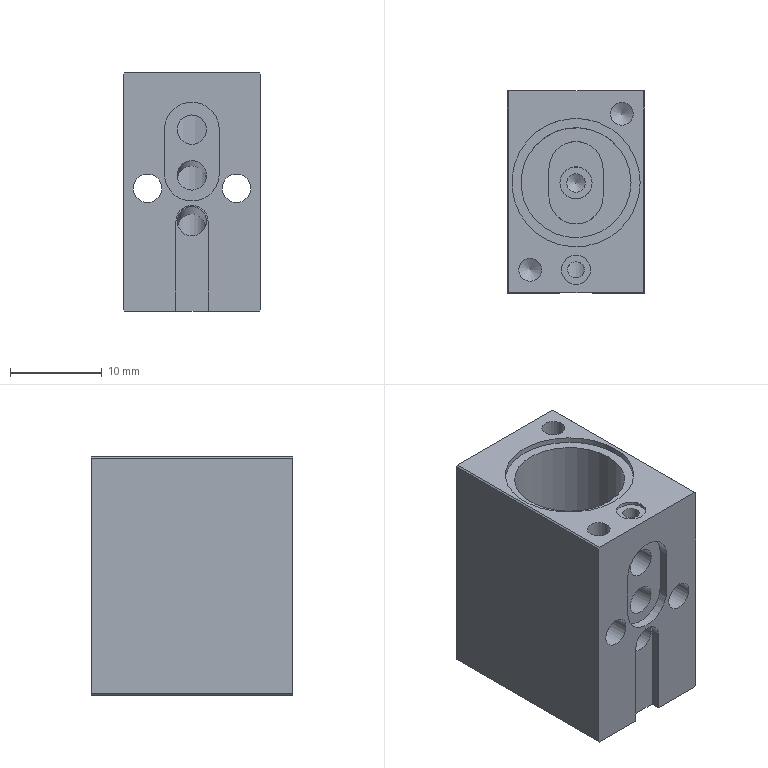NC program | NX | posted with a generic post | part box 15 x 22 x 26 mm
Whole program:
N10 G17 G21 G94 G90
(PLANAR_MILL_13 , TOOL : D8开粗)
N12 T13 M6
N14 G54
N16 G17 G0 G90 X-19. Y-18. B0. C0. S5500 M3
N18 G43 Z30. H13
N20 Z5.
N22 G94 G1 Z2. F1000.
N24 Y-10.
N26 Y10.
N28 Y18.
N30 Z5.
N32 G0 Z30.
N34 Y-18.
N36 Z4.
N38 G1 Z1.
N40 Y-10.
N42 Y10.
N44 Y18.
N46 Z4.
N48 G0 Z30.
N50 Y-18.
N52 Z3.
N54 G1 Z0.
N56 Y-10.
N58 Y10.
N60 Y18.
N62 Z3.
N64 G0 Z30.
(ADAPTIVE_MILLING_1 , TOOL : D8开粗)
N66 X24.104 Y0.904
N68 Z3.
N70 G1 X23.955 Y0.889 Z2.063 F3000.
N72 X23.806 Y0.873 Z1.692
N74 X23.656 Y0.858 Z1.42
N76 X23.507 Y0.843 Z1.2
N78 X23.358 Y0.827 Z1.016
N80 X23.209 Y0.812 Z0.858
N82 X23.06 Y0.796 Z0.72
N84 X22.91 Y0.781 Z0.6
N86 X22.761 Y0.765 Z0.495
N88 X22.612 Y0.75 Z0.402
N90 X22.463 Y0.734 Z0.321
N92 X22.314 Y0.719 Z0.25
N94 X22.164 Y0.704 Z0.19
N96 X22.015 Y0.688 Z0.138
N98 X21.866 Y0.673 Z0.095
N100 X21.717 Y0.657 Z0.061
N102 X21.568 Y0.642 Z0.034
N104 X21.418 Y0.626 Z0.015
N106 X21.269 Y0.611 Z0.004
N108 X21.12 Y0.596 Z0.
N110 X19.694 Y0.448
N112 G3 X19.077 Y0.048 R0.81
N114 X18.556 Y-1.641 R4.483
N116 X18.231 Y-7.12 R41.154
N118 G2 X16.258 Y-11.16 R4.599
N120 X12.294 Y-12.725 R9.323
N122 X6.516 Y-13.155 R38.101
N124 X-2.884 Y-13.197 R675.849
N126 X-12.875 Y-13.18 R776.549
N128 X-16.074 Y-11.344 R4.516
N130 X-17.679 Y-7.505 R8.936
N132 X-18.147 Y-1.831 R34.624
N134 X-18.181 Y7.869 R519.831
N136 X-16.348 Y11.069 R4.511
N138 X-12.507 Y12.676 R8.947
N140 X-6.834 Y13.147 R34.39
N142 X3.066 Y13.197 R678.674
N144 G1 X12.839 Y13.183
N146 G2 X16.05 Y11.37 R4.506
N148 X17.671 Y7.537 R8.889
N150 X18.054 Y1.465 R24.421
N152 G3 X17.467 Y-5.897 R123.751
N154 G2 X14.688 Y-10.215 R6.118
N156 X10.219 Y-11.873 R11.431
N158 X3.743 Y-12.351 R43.566
N160 X-10.675 Y-12.381 R782.589
N162 X-15.105 Y-9.775 R5.952
N164 X-16.84 Y-5.341 R10.993
N166 X-17.341 Y0.833 R39.75
N168 X-17.363 Y5.831 R77.968
N170 X-14.734 Y10.13 R5.975
N172 X-10.292 Y11.847 R11.055
N174 X-4.118 Y12.342 R40.333
N176 X10.671 Y12.381 R778.316
N178 X15.046 Y9.852 R5.924
N180 X16.821 Y5.426 R10.766
N182 X17.023 Y0.342 R21.503
N184 X16.744 Y-4.139 R151.437
N186 X13.189 Y-9.448 R7.178
N188 X8.186 Y-11.106 R13.584
N190 X1.706 Y-11.547 R50.699
N192 X-8.793 Y-11.578 R473.295
N194 X-14.32 Y-8.27 R6.93
N196 X-16.055 Y-3.402 R12.851
N198 X-16.514 Y4.074 R41.876
N200 X-13.337 Y9.265 R6.833
N202 X-8.583 Y11.021 R12.467
N204 X-2.109 Y11.536 R43.77
N206 X8.79 Y11.578 R447.107
N208 X14.322 Y8.267 R6.923
N210 X15.975 Y3.061 R11.541
N212 X15.927 Y-2.929 R30.282
N214 X12.071 Y-8.533 R7.798
N216 X6.979 Y-10.245 R14.273
N218 X-0.097 Y-10.745 R51.827
N220 X-7.197 Y-10.768 R184.855
N222 X-13.565 Y-6.867 R7.642
N224 X-15.274 Y-1.674 R14.415
N226 X-15.59 Y2.608 R22.392
N228 X-12.093 Y8.386 R7.332
N230 X-7.241 Y10.17 R13.211
N232 X-0.471 Y10.73 R44.785
N234 X7.328 Y10.76 R147.638
N236 X13.745 Y6.466 R7.571
N238 X15.039 Y1.456 R13.612
N240 X14.857 Y-2.621 R12.422
N242 X10.804 Y-7.752 R8.196
N244 X5.592 Y-9.435 R15.35
N246 X-1.784 Y-9.945 R55.309
N248 X-6.182 Y-9.921 R50.932
N250 X-12.677 Y-5.776 R8.127
N252 X-14.544 Y1.408 R14.733
N254 X-11.22 Y7.302 R7.467
N256 X-6.327 Y9.26 R13.02
N258 X0.534 Y9.91 R41.3
N260 X6.033 Y9.933 R70.86
N262 X12.763 Y5.43 R7.885
N264 X13.961 Y-0.774 R11.562
N266 X10.313 Y-6.506 R7.964
N268 X5.11 Y-8.481 R14.106
N270 X-2.156 Y-9.117 R46.337
N272 X-6.043 Y-8.932 R17.987
N274 X-11.876 Y-4.605 R8.528
N276 X-13.334 Y0.433 R10.475
N278 X-10.341 Y6.202 R7.294
N280 X-5.424 Y8.351 R12.556
N282 X1.127 Y9.075 R36.823
N284 X5.422 Y9.03 R27.597
N286 X11.791 Y4.428 R8.098
N288 X12.513 Y-1.104 R7.974
N290 X9.022 Y-5.74 R7.923
N292 X3.798 Y-7.679 R14.473
N294 X-3.768 Y-8.218 R34.051
N296 X-11.855 Y-1.115 R8.684
N298 X-9.591 Y4.901 R6.747
N300 X-4.81 Y7.358 R11.364
N302 X3.719 Y8.212 R30.843
N304 X10.508 Y3.943 R8.036
N306 X9.547 Y-3.334 R6.47
N308 X5.211 Y-6.151 R10.108
N310 X-2.964 Y-7.28 R22.183
N312 X-9.193 Y-3.925 R8.358
N314 X-9.086 Y2.997 R5.85
N316 X-4.945 Y6.037 R9.086
N318 X3.007 Y7.249 R19.839
N320 X7.923 Y5.052 R7.618
N322 X8.581 Y-1.693 R5.51
N324 X4.734 Y-4.954 R8.487
N326 X-2.277 Y-6.257 R14.992
N328 X-6.522 Y-4.653 R7.635
N330 X-7.785 Y1.354 R4.951
N332 X-4.533 Y4.659 R7.475
N334 X2.412 Y6.168 R12.721
N336 X5.717 Y4.888 R5.886
N338 X6.993 Y0.054 R4.51
N340 X4.015 Y-3.589 R6.799
N342 X-2.303 Y-4.996 R9.455
N344 X-5.671 Y-0.574 R3.864
N346 X-3.329 Y3.244 R5.788
N348 X1.119 Y4.808 R7.302
N350 X3.829 Y2.401 R2.967
N352 X2.639 Y-1.561 R4.489
N354 G1 X1.887 Y-2.363
N356 X1.786 Y-2.474 Z0.004
N358 X1.685 Y-2.585 Z0.015
N360 X1.584 Y-2.696 Z0.034
N362 X1.483 Y-2.807 Z0.061
N364 X1.382 Y-2.918 Z0.095
N366 X1.281 Y-3.028 Z0.138
N368 X1.18 Y-3.139 Z0.19
N370 X1.079 Y-3.25 Z0.25
N372 X0.978 Y-3.361 Z0.321
N374 X0.877 Y-3.472 Z0.402
N376 X0.776 Y-3.583 Z0.495
N378 X0.675 Y-3.694 Z0.6
N380 X0.574 Y-3.805 Z0.72
N382 X0.473 Y-3.916 Z0.858
N384 X0.372 Y-4.027 Z1.016
N386 X0.271 Y-4.138 Z1.2
N388 X0.17 Y-4.248 Z1.42
N390 X0.069 Y-4.359 Z1.692
N392 X-0.032 Y-4.47 Z2.063
N394 X-0.133 Y-4.581 Z3.
N396 G0 Z30.
N398 M5
(PLANAR_MILL_14 , TOOL : D50面刀)
N400 T12 M6
N402 G54
N404 G17 G0 G90 X41. Y-0.5 B0. C0. S4000 M3
N406 G43 Z30. H12
N408 Z2.
N410 G94 G1 Z0. F800.
N412 X13.
N414 X-13.
N416 X-41.
N418 Z2.
N420 G0 Z30.
N422 M5
(PLANAR_MILL_15 , TOOL : D3点钻)
N424 T06 M6
N426 G54
N428 G17 G0 G90 X14.951 Y-9.571 B0. C0. S4500 M3
N430 G43 Z30. H6
N432 Z1.
N434 G94 G1 Z-1. F1000.
N436 X13.536 Y-8.157
N438 G2 X12.829 Y-8.45 R1.
N440 G1 X-12.829
N442 G2 X-13.536 Y-8.157 R1.
N444 G1 X-13.657 Y-8.036
N446 G2 X-13.95 Y-7.329 R1.
N448 G1 Y7.329
N450 G2 X-13.657 Y8.036 R1.
N452 G1 X-13.536 Y8.157
N454 G2 X-12.829 Y8.45 R1.
N456 G1 X12.829
N458 G2 X13.536 Y8.157 R1.
N460 G1 X13.657 Y8.036
N462 G2 X13.95 Y7.329 R1.
N464 G1 Y-7.329
N466 G2 X13.657 Y-8.036 R1.
N468 G1 X13.536 Y-8.157
N470 X14.951 Y-9.571
N472 Z1.
N474 G0 Z30.
(PLANAR_MILL_16 , TOOL : D3点钻)
N476 X-0.003 Y5.05
N478 Z1.
N480 G1 Z-1. F600.
N482 X-0.05
N484 G3 X-0.25 Y4.85 R0.2
N486 X0.4 Y4.2 R0.65
N488 X-0.25 Y4.85 R-0.65
N490 X-0.05 Y4.65 R0.2
N492 G1 X-0.003
N494 Z1.
N496 G0 Z30.
N498 X0.803 Y-5.05
N500 Z1.
N502 G1 Z-1.
N504 X0.85
N506 G3 X1.05 Y-4.85 R0.2
N508 X0.4 Y-4.2 R0.65
N510 X1.05 Y-4.85 R-0.65
N512 X0.85 Y-4.65 R0.2
N514 G1 X0.803
N516 Z1.
N518 G0 Z30.
N520 M5
N522 M2